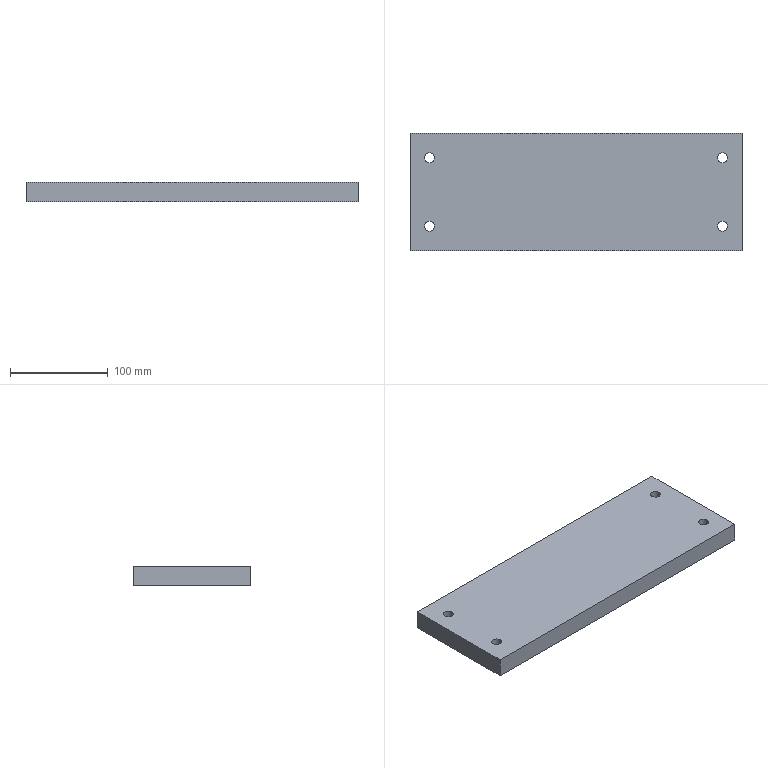Part | SolidWorks | features Extrusion 1 | 1 solid | 14 faces | box 340 x 120 x 20 mm | volume 809717 mm3 | cylinder 8 | plane 6 | commonest cylinder face diameters 10 x8
STEP:
#1=CARTESIAN_POINT('',(15.,25.,20.));
#2=VERTEX_POINT('',#1);
#3=CARTESIAN_POINT('',(25.,25.,20.));
#4=VERTEX_POINT('',#3);
#5=CARTESIAN_POINT('',(20.,25.,20.));
#6=DIRECTION('',(0.,0.,1.));
#7=DIRECTION('',(1.,0.,0.));
#8=AXIS2_PLACEMENT_3D('',#5,#6,#7);
#9=CIRCLE('',#8,5.);
#10=EDGE_CURVE('',#2,#4,#9,.T.);
#11=ORIENTED_EDGE('',*,*,#10,.T.);
#12=CARTESIAN_POINT('',(25.,25.,0.));
#13=VERTEX_POINT('',#12);
#14=CARTESIAN_POINT('',(25.,25.,20.));
#15=DIRECTION('',(0.,0.,-1.));
#16=VECTOR('',#15,1000.);
#17=LINE('',#14,#16);
#18=EDGE_CURVE('',#4,#13,#17,.T.);
#19=ORIENTED_EDGE('',*,*,#18,.T.);
#20=CARTESIAN_POINT('',(15.,25.,0.));
#21=VERTEX_POINT('',#20);
#22=CARTESIAN_POINT('',(20.,25.,0.));
#23=DIRECTION('',(0.,0.,1.));
#24=DIRECTION('',(1.,0.,0.));
#25=AXIS2_PLACEMENT_3D('',#22,#23,#24);
#26=CIRCLE('',#25,5.);
#27=EDGE_CURVE('',#21,#13,#26,.T.);
#28=ORIENTED_EDGE('',*,*,#27,.F.);
#29=CARTESIAN_POINT('',(15.,25.,20.));
#30=DIRECTION('',(0.,0.,-1.));
#31=VECTOR('',#30,1000.);
#32=LINE('',#29,#31);
#33=EDGE_CURVE('',#2,#21,#32,.T.);
#34=ORIENTED_EDGE('',*,*,#33,.F.);
#35=EDGE_LOOP('',(#11,#19,#28,#34));
#36=FACE_OUTER_BOUND('',#35,.T.);
#37=CARTESIAN_POINT('',(20.,25.,20.));
#38=DIRECTION('',(0.,0.,-1.));
#39=DIRECTION('',(-1.,0.,0.));
#40=AXIS2_PLACEMENT_3D('',#37,#38,#39);
#41=CYLINDRICAL_SURFACE('',#40,5.);
#42=ADVANCED_FACE('',(#36),#41,.F.);
#43=CARTESIAN_POINT('',(315.,25.,20.));
#44=VERTEX_POINT('',#43);
#45=CARTESIAN_POINT('',(325.,25.,20.));
#46=VERTEX_POINT('',#45);
#47=CARTESIAN_POINT('',(320.,25.,20.));
#48=DIRECTION('',(0.,0.,1.));
#49=DIRECTION('',(1.,0.,0.));
#50=AXIS2_PLACEMENT_3D('',#47,#48,#49);
#51=CIRCLE('',#50,5.);
#52=EDGE_CURVE('',#44,#46,#51,.T.);
#53=ORIENTED_EDGE('',*,*,#52,.T.);
#54=CARTESIAN_POINT('',(325.,25.,0.));
#55=VERTEX_POINT('',#54);
#56=CARTESIAN_POINT('',(325.,25.,20.));
#57=DIRECTION('',(0.,0.,-1.));
#58=VECTOR('',#57,1000.);
#59=LINE('',#56,#58);
#60=EDGE_CURVE('',#46,#55,#59,.T.);
#61=ORIENTED_EDGE('',*,*,#60,.T.);
#62=CARTESIAN_POINT('',(315.,25.,0.));
#63=VERTEX_POINT('',#62);
#64=CARTESIAN_POINT('',(320.,25.,0.));
#65=DIRECTION('',(0.,0.,1.));
#66=DIRECTION('',(1.,0.,0.));
#67=AXIS2_PLACEMENT_3D('',#64,#65,#66);
#68=CIRCLE('',#67,5.);
#69=EDGE_CURVE('',#63,#55,#68,.T.);
#70=ORIENTED_EDGE('',*,*,#69,.F.);
#71=CARTESIAN_POINT('',(315.,25.,20.));
#72=DIRECTION('',(0.,0.,-1.));
#73=VECTOR('',#72,1000.);
#74=LINE('',#71,#73);
#75=EDGE_CURVE('',#44,#63,#74,.T.);
#76=ORIENTED_EDGE('',*,*,#75,.F.);
#77=EDGE_LOOP('',(#53,#61,#70,#76));
#78=FACE_OUTER_BOUND('',#77,.T.);
#79=CARTESIAN_POINT('',(320.,25.,20.));
#80=DIRECTION('',(0.,0.,-1.));
#81=DIRECTION('',(-1.,0.,0.));
#82=AXIS2_PLACEMENT_3D('',#79,#80,#81);
#83=CYLINDRICAL_SURFACE('',#82,5.);
#84=ADVANCED_FACE('',(#78),#83,.F.);
#85=CARTESIAN_POINT('',(315.,95.,20.));
#86=VERTEX_POINT('',#85);
#87=CARTESIAN_POINT('',(325.,95.,20.));
#88=VERTEX_POINT('',#87);
#89=CARTESIAN_POINT('',(320.,95.,20.));
#90=DIRECTION('',(0.,0.,1.));
#91=DIRECTION('',(1.,0.,0.));
#92=AXIS2_PLACEMENT_3D('',#89,#90,#91);
#93=CIRCLE('',#92,5.);
#94=EDGE_CURVE('',#86,#88,#93,.T.);
#95=ORIENTED_EDGE('',*,*,#94,.T.);
#96=CARTESIAN_POINT('',(325.,95.,0.));
#97=VERTEX_POINT('',#96);
#98=CARTESIAN_POINT('',(325.,95.,20.));
#99=DIRECTION('',(0.,0.,-1.));
#100=VECTOR('',#99,1000.);
#101=LINE('',#98,#100);
#102=EDGE_CURVE('',#88,#97,#101,.T.);
#103=ORIENTED_EDGE('',*,*,#102,.T.);
#104=CARTESIAN_POINT('',(315.,95.,0.));
#105=VERTEX_POINT('',#104);
#106=CARTESIAN_POINT('',(320.,95.,0.));
#107=DIRECTION('',(0.,0.,1.));
#108=DIRECTION('',(1.,0.,0.));
#109=AXIS2_PLACEMENT_3D('',#106,#107,#108);
#110=CIRCLE('',#109,5.);
#111=EDGE_CURVE('',#105,#97,#110,.T.);
#112=ORIENTED_EDGE('',*,*,#111,.F.);
#113=CARTESIAN_POINT('',(315.,95.,20.));
#114=DIRECTION('',(0.,0.,-1.));
#115=VECTOR('',#114,1000.);
#116=LINE('',#113,#115);
#117=EDGE_CURVE('',#86,#105,#116,.T.);
#118=ORIENTED_EDGE('',*,*,#117,.F.);
#119=EDGE_LOOP('',(#95,#103,#112,#118));
#120=FACE_OUTER_BOUND('',#119,.T.);
#121=CARTESIAN_POINT('',(320.,95.,20.));
#122=DIRECTION('',(0.,0.,-1.));
#123=DIRECTION('',(-1.,0.,0.));
#124=AXIS2_PLACEMENT_3D('',#121,#122,#123);
#125=CYLINDRICAL_SURFACE('',#124,5.);
#126=ADVANCED_FACE('',(#120),#125,.F.);
#127=CARTESIAN_POINT('',(15.,95.,20.));
#128=VERTEX_POINT('',#127);
#129=CARTESIAN_POINT('',(25.,95.,20.));
#130=VERTEX_POINT('',#129);
#131=CARTESIAN_POINT('',(20.,95.,20.));
#132=DIRECTION('',(0.,0.,1.));
#133=DIRECTION('',(1.,0.,0.));
#134=AXIS2_PLACEMENT_3D('',#131,#132,#133);
#135=CIRCLE('',#134,5.);
#136=EDGE_CURVE('',#128,#130,#135,.T.);
#137=ORIENTED_EDGE('',*,*,#136,.T.);
#138=CARTESIAN_POINT('',(25.,95.,0.));
#139=VERTEX_POINT('',#138);
#140=CARTESIAN_POINT('',(25.,95.,20.));
#141=DIRECTION('',(0.,0.,-1.));
#142=VECTOR('',#141,1000.);
#143=LINE('',#140,#142);
#144=EDGE_CURVE('',#130,#139,#143,.T.);
#145=ORIENTED_EDGE('',*,*,#144,.T.);
#146=CARTESIAN_POINT('',(15.,95.,0.));
#147=VERTEX_POINT('',#146);
#148=CARTESIAN_POINT('',(20.,95.,0.));
#149=DIRECTION('',(0.,0.,1.));
#150=DIRECTION('',(1.,0.,0.));
#151=AXIS2_PLACEMENT_3D('',#148,#149,#150);
#152=CIRCLE('',#151,5.);
#153=EDGE_CURVE('',#147,#139,#152,.T.);
#154=ORIENTED_EDGE('',*,*,#153,.F.);
#155=CARTESIAN_POINT('',(15.,95.,20.));
#156=DIRECTION('',(0.,0.,-1.));
#157=VECTOR('',#156,1000.);
#158=LINE('',#155,#157);
#159=EDGE_CURVE('',#128,#147,#158,.T.);
#160=ORIENTED_EDGE('',*,*,#159,.F.);
#161=EDGE_LOOP('',(#137,#145,#154,#160));
#162=FACE_OUTER_BOUND('',#161,.T.);
#163=CARTESIAN_POINT('',(20.,95.,20.));
#164=DIRECTION('',(0.,0.,-1.));
#165=DIRECTION('',(-1.,0.,0.));
#166=AXIS2_PLACEMENT_3D('',#163,#164,#165);
#167=CYLINDRICAL_SURFACE('',#166,5.);
#168=ADVANCED_FACE('',(#162),#167,.F.);
#169=CARTESIAN_POINT('',(0.,120.,20.));
#170=VERTEX_POINT('',#169);
#171=CARTESIAN_POINT('',(0.,0.,20.));
#172=VERTEX_POINT('',#171);
#173=CARTESIAN_POINT('',(0.,0.,20.));
#174=DIRECTION('',(0.,-1.,0.));
#175=VECTOR('',#174,1000.);
#176=LINE('',#173,#175);
#177=EDGE_CURVE('',#170,#172,#176,.T.);
#178=ORIENTED_EDGE('',*,*,#177,.T.);
#179=CARTESIAN_POINT('',(340.,0.,20.));
#180=VERTEX_POINT('',#179);
#181=CARTESIAN_POINT('',(0.,0.,20.));
#182=DIRECTION('',(1.,0.,0.));
#183=VECTOR('',#182,1000.);
#184=LINE('',#181,#183);
#185=EDGE_CURVE('',#172,#180,#184,.T.);
#186=ORIENTED_EDGE('',*,*,#185,.T.);
#187=CARTESIAN_POINT('',(340.,120.,20.));
#188=VERTEX_POINT('',#187);
#189=CARTESIAN_POINT('',(340.,0.,20.));
#190=DIRECTION('',(0.,1.,0.));
#191=VECTOR('',#190,1000.);
#192=LINE('',#189,#191);
#193=EDGE_CURVE('',#180,#188,#192,.T.);
#194=ORIENTED_EDGE('',*,*,#193,.T.);
#195=CARTESIAN_POINT('',(0.,120.,20.));
#196=DIRECTION('',(-1.,0.,0.));
#197=VECTOR('',#196,1000.);
#198=LINE('',#195,#197);
#199=EDGE_CURVE('',#188,#170,#198,.T.);
#200=ORIENTED_EDGE('',*,*,#199,.T.);
#201=EDGE_LOOP('',(#178,#186,#194,#200));
#202=FACE_OUTER_BOUND('',#201,.T.);
#203=ORIENTED_EDGE('',*,*,#136,.F.);
#204=CARTESIAN_POINT('',(20.,95.,20.));
#205=DIRECTION('',(0.,0.,1.));
#206=DIRECTION('',(1.,0.,0.));
#207=AXIS2_PLACEMENT_3D('',#204,#205,#206);
#208=CIRCLE('',#207,5.);
#209=EDGE_CURVE('',#130,#128,#208,.T.);
#210=ORIENTED_EDGE('',*,*,#209,.F.);
#211=EDGE_LOOP('',(#203,#210));
#212=FACE_BOUND('',#211,.T.);
#213=ORIENTED_EDGE('',*,*,#94,.F.);
#214=CARTESIAN_POINT('',(320.,95.,20.));
#215=DIRECTION('',(0.,0.,1.));
#216=DIRECTION('',(1.,0.,0.));
#217=AXIS2_PLACEMENT_3D('',#214,#215,#216);
#218=CIRCLE('',#217,5.);
#219=EDGE_CURVE('',#88,#86,#218,.T.);
#220=ORIENTED_EDGE('',*,*,#219,.F.);
#221=EDGE_LOOP('',(#213,#220));
#222=FACE_BOUND('',#221,.T.);
#223=ORIENTED_EDGE('',*,*,#52,.F.);
#224=CARTESIAN_POINT('',(320.,25.,20.));
#225=DIRECTION('',(0.,0.,1.));
#226=DIRECTION('',(1.,0.,0.));
#227=AXIS2_PLACEMENT_3D('',#224,#225,#226);
#228=CIRCLE('',#227,5.);
#229=EDGE_CURVE('',#46,#44,#228,.T.);
#230=ORIENTED_EDGE('',*,*,#229,.F.);
#231=EDGE_LOOP('',(#223,#230));
#232=FACE_BOUND('',#231,.T.);
#233=ORIENTED_EDGE('',*,*,#10,.F.);
#234=CARTESIAN_POINT('',(20.,25.,20.));
#235=DIRECTION('',(0.,0.,1.));
#236=DIRECTION('',(1.,0.,0.));
#237=AXIS2_PLACEMENT_3D('',#234,#235,#236);
#238=CIRCLE('',#237,5.);
#239=EDGE_CURVE('',#4,#2,#238,.T.);
#240=ORIENTED_EDGE('',*,*,#239,.F.);
#241=EDGE_LOOP('',(#233,#240));
#242=FACE_BOUND('',#241,.T.);
#243=CARTESIAN_POINT('',(0.,0.,20.));
#244=DIRECTION('',(0.,0.,-1.));
#245=DIRECTION('',(-1.,0.,0.));
#246=AXIS2_PLACEMENT_3D('',#243,#244,#245);
#247=PLANE('',#246);
#248=ADVANCED_FACE('',(#202,#212,#222,#232,#242),#247,.F.);
#249=ORIENTED_EDGE('',*,*,#69,.T.);
#250=CARTESIAN_POINT('',(320.,25.,0.));
#251=DIRECTION('',(0.,0.,1.));
#252=DIRECTION('',(1.,0.,0.));
#253=AXIS2_PLACEMENT_3D('',#250,#251,#252);
#254=CIRCLE('',#253,5.);
#255=EDGE_CURVE('',#55,#63,#254,.T.);
#256=ORIENTED_EDGE('',*,*,#255,.T.);
#257=EDGE_LOOP('',(#249,#256));
#258=FACE_BOUND('',#257,.T.);
#259=ORIENTED_EDGE('',*,*,#153,.T.);
#260=CARTESIAN_POINT('',(20.,95.,0.));
#261=DIRECTION('',(0.,0.,1.));
#262=DIRECTION('',(1.,0.,0.));
#263=AXIS2_PLACEMENT_3D('',#260,#261,#262);
#264=CIRCLE('',#263,5.);
#265=EDGE_CURVE('',#139,#147,#264,.T.);
#266=ORIENTED_EDGE('',*,*,#265,.T.);
#267=EDGE_LOOP('',(#259,#266));
#268=FACE_BOUND('',#267,.T.);
#269=CARTESIAN_POINT('',(0.,120.,0.));
#270=VERTEX_POINT('',#269);
#271=CARTESIAN_POINT('',(0.,0.,0.));
#272=VERTEX_POINT('',#271);
#273=CARTESIAN_POINT('',(0.,0.,0.));
#274=DIRECTION('',(0.,-1.,0.));
#275=VECTOR('',#274,1000.);
#276=LINE('',#273,#275);
#277=EDGE_CURVE('',#270,#272,#276,.T.);
#278=ORIENTED_EDGE('',*,*,#277,.F.);
#279=CARTESIAN_POINT('',(340.,120.,0.));
#280=VERTEX_POINT('',#279);
#281=CARTESIAN_POINT('',(0.,120.,0.));
#282=DIRECTION('',(-1.,0.,0.));
#283=VECTOR('',#282,1000.);
#284=LINE('',#281,#283);
#285=EDGE_CURVE('',#280,#270,#284,.T.);
#286=ORIENTED_EDGE('',*,*,#285,.F.);
#287=CARTESIAN_POINT('',(340.,0.,0.));
#288=VERTEX_POINT('',#287);
#289=CARTESIAN_POINT('',(340.,0.,0.));
#290=DIRECTION('',(0.,1.,0.));
#291=VECTOR('',#290,1000.);
#292=LINE('',#289,#291);
#293=EDGE_CURVE('',#288,#280,#292,.T.);
#294=ORIENTED_EDGE('',*,*,#293,.F.);
#295=CARTESIAN_POINT('',(0.,0.,0.));
#296=DIRECTION('',(1.,0.,0.));
#297=VECTOR('',#296,1000.);
#298=LINE('',#295,#297);
#299=EDGE_CURVE('',#272,#288,#298,.T.);
#300=ORIENTED_EDGE('',*,*,#299,.F.);
#301=EDGE_LOOP('',(#278,#286,#294,#300));
#302=FACE_OUTER_BOUND('',#301,.T.);
#303=ORIENTED_EDGE('',*,*,#111,.T.);
#304=CARTESIAN_POINT('',(320.,95.,0.));
#305=DIRECTION('',(0.,0.,1.));
#306=DIRECTION('',(1.,0.,0.));
#307=AXIS2_PLACEMENT_3D('',#304,#305,#306);
#308=CIRCLE('',#307,5.);
#309=EDGE_CURVE('',#97,#105,#308,.T.);
#310=ORIENTED_EDGE('',*,*,#309,.T.);
#311=EDGE_LOOP('',(#303,#310));
#312=FACE_BOUND('',#311,.T.);
#313=ORIENTED_EDGE('',*,*,#27,.T.);
#314=CARTESIAN_POINT('',(20.,25.,0.));
#315=DIRECTION('',(0.,0.,1.));
#316=DIRECTION('',(1.,0.,0.));
#317=AXIS2_PLACEMENT_3D('',#314,#315,#316);
#318=CIRCLE('',#317,5.);
#319=EDGE_CURVE('',#13,#21,#318,.T.);
#320=ORIENTED_EDGE('',*,*,#319,.T.);
#321=EDGE_LOOP('',(#313,#320));
#322=FACE_BOUND('',#321,.T.);
#323=CARTESIAN_POINT('',(0.,0.,0.));
#324=DIRECTION('',(0.,0.,-1.));
#325=DIRECTION('',(-1.,0.,0.));
#326=AXIS2_PLACEMENT_3D('',#323,#324,#325);
#327=PLANE('',#326);
#328=ADVANCED_FACE('',(#258,#268,#302,#312,#322),#327,.T.);
#329=ORIENTED_EDGE('',*,*,#277,.T.);
#330=CARTESIAN_POINT('',(0.,0.,20.));
#331=DIRECTION('',(0.,0.,-1.));
#332=VECTOR('',#331,1000.);
#333=LINE('',#330,#332);
#334=EDGE_CURVE('',#172,#272,#333,.T.);
#335=ORIENTED_EDGE('',*,*,#334,.F.);
#336=ORIENTED_EDGE('',*,*,#177,.F.);
#337=CARTESIAN_POINT('',(0.,120.,20.));
#338=DIRECTION('',(0.,0.,-1.));
#339=VECTOR('',#338,1000.);
#340=LINE('',#337,#339);
#341=EDGE_CURVE('',#170,#270,#340,.T.);
#342=ORIENTED_EDGE('',*,*,#341,.T.);
#343=EDGE_LOOP('',(#329,#335,#336,#342));
#344=FACE_OUTER_BOUND('',#343,.T.);
#345=CARTESIAN_POINT('',(0.,0.,20.));
#346=DIRECTION('',(1.,0.,0.));
#347=DIRECTION('',(0.,0.,-1.));
#348=AXIS2_PLACEMENT_3D('',#345,#346,#347);
#349=PLANE('',#348);
#350=ADVANCED_FACE('',(#344),#349,.F.);
#351=ORIENTED_EDGE('',*,*,#299,.T.);
#352=CARTESIAN_POINT('',(340.,0.,20.));
#353=DIRECTION('',(0.,0.,-1.));
#354=VECTOR('',#353,1000.);
#355=LINE('',#352,#354);
#356=EDGE_CURVE('',#180,#288,#355,.T.);
#357=ORIENTED_EDGE('',*,*,#356,.F.);
#358=ORIENTED_EDGE('',*,*,#185,.F.);
#359=ORIENTED_EDGE('',*,*,#334,.T.);
#360=EDGE_LOOP('',(#351,#357,#358,#359));
#361=FACE_OUTER_BOUND('',#360,.T.);
#362=CARTESIAN_POINT('',(0.,0.,20.));
#363=DIRECTION('',(0.,1.,0.));
#364=DIRECTION('',(0.,0.,1.));
#365=AXIS2_PLACEMENT_3D('',#362,#363,#364);
#366=PLANE('',#365);
#367=ADVANCED_FACE('',(#361),#366,.F.);
#368=ORIENTED_EDGE('',*,*,#293,.T.);
#369=CARTESIAN_POINT('',(340.,120.,20.));
#370=DIRECTION('',(0.,0.,-1.));
#371=VECTOR('',#370,1000.);
#372=LINE('',#369,#371);
#373=EDGE_CURVE('',#188,#280,#372,.T.);
#374=ORIENTED_EDGE('',*,*,#373,.F.);
#375=ORIENTED_EDGE('',*,*,#193,.F.);
#376=ORIENTED_EDGE('',*,*,#356,.T.);
#377=EDGE_LOOP('',(#368,#374,#375,#376));
#378=FACE_OUTER_BOUND('',#377,.T.);
#379=CARTESIAN_POINT('',(340.,0.,20.));
#380=DIRECTION('',(-1.,0.,0.));
#381=DIRECTION('',(0.,0.,1.));
#382=AXIS2_PLACEMENT_3D('',#379,#380,#381);
#383=PLANE('',#382);
#384=ADVANCED_FACE('',(#378),#383,.F.);
#385=ORIENTED_EDGE('',*,*,#285,.T.);
#386=ORIENTED_EDGE('',*,*,#341,.F.);
#387=ORIENTED_EDGE('',*,*,#199,.F.);
#388=ORIENTED_EDGE('',*,*,#373,.T.);
#389=EDGE_LOOP('',(#385,#386,#387,#388));
#390=FACE_OUTER_BOUND('',#389,.T.);
#391=CARTESIAN_POINT('',(0.,120.,20.));
#392=DIRECTION('',(0.,-1.,0.));
#393=DIRECTION('',(0.,0.,-1.));
#394=AXIS2_PLACEMENT_3D('',#391,#392,#393);
#395=PLANE('',#394);
#396=ADVANCED_FACE('',(#390),#395,.F.);
#397=ORIENTED_EDGE('',*,*,#144,.F.);
#398=ORIENTED_EDGE('',*,*,#209,.T.);
#399=ORIENTED_EDGE('',*,*,#159,.T.);
#400=ORIENTED_EDGE('',*,*,#265,.F.);
#401=EDGE_LOOP('',(#397,#398,#399,#400));
#402=FACE_OUTER_BOUND('',#401,.T.);
#403=CARTESIAN_POINT('',(20.,95.,20.));
#404=DIRECTION('',(0.,0.,-1.));
#405=DIRECTION('',(-1.,0.,0.));
#406=AXIS2_PLACEMENT_3D('',#403,#404,#405);
#407=CYLINDRICAL_SURFACE('',#406,5.);
#408=ADVANCED_FACE('',(#402),#407,.F.);
#409=ORIENTED_EDGE('',*,*,#102,.F.);
#410=ORIENTED_EDGE('',*,*,#219,.T.);
#411=ORIENTED_EDGE('',*,*,#117,.T.);
#412=ORIENTED_EDGE('',*,*,#309,.F.);
#413=EDGE_LOOP('',(#409,#410,#411,#412));
#414=FACE_OUTER_BOUND('',#413,.T.);
#415=CARTESIAN_POINT('',(320.,95.,20.));
#416=DIRECTION('',(0.,0.,-1.));
#417=DIRECTION('',(-1.,0.,0.));
#418=AXIS2_PLACEMENT_3D('',#415,#416,#417);
#419=CYLINDRICAL_SURFACE('',#418,5.);
#420=ADVANCED_FACE('',(#414),#419,.F.);
#421=ORIENTED_EDGE('',*,*,#60,.F.);
#422=ORIENTED_EDGE('',*,*,#229,.T.);
#423=ORIENTED_EDGE('',*,*,#75,.T.);
#424=ORIENTED_EDGE('',*,*,#255,.F.);
#425=EDGE_LOOP('',(#421,#422,#423,#424));
#426=FACE_OUTER_BOUND('',#425,.T.);
#427=CARTESIAN_POINT('',(320.,25.,20.));
#428=DIRECTION('',(0.,0.,-1.));
#429=DIRECTION('',(-1.,0.,0.));
#430=AXIS2_PLACEMENT_3D('',#427,#428,#429);
#431=CYLINDRICAL_SURFACE('',#430,5.);
#432=ADVANCED_FACE('',(#426),#431,.F.);
#433=ORIENTED_EDGE('',*,*,#18,.F.);
#434=ORIENTED_EDGE('',*,*,#239,.T.);
#435=ORIENTED_EDGE('',*,*,#33,.T.);
#436=ORIENTED_EDGE('',*,*,#319,.F.);
#437=EDGE_LOOP('',(#433,#434,#435,#436));
#438=FACE_OUTER_BOUND('',#437,.T.);
#439=CARTESIAN_POINT('',(20.,25.,20.));
#440=DIRECTION('',(0.,0.,-1.));
#441=DIRECTION('',(-1.,0.,0.));
#442=AXIS2_PLACEMENT_3D('',#439,#440,#441);
#443=CYLINDRICAL_SURFACE('',#442,5.);
#444=ADVANCED_FACE('',(#438),#443,.F.);
#445=CLOSED_SHELL('',(#42,#84,#126,#168,#248,#328,#350,#367,#384,#396,#408,#420,#432,#444));
#446=MANIFOLD_SOLID_BREP('',#445);
#447=CARTESIAN_POINT('',(0.,0.,0.));
#448=DIRECTION('',(0.,0.,1.));
#449=DIRECTION('',(1.,0.,0.));
#450=AXIS2_PLACEMENT_3D('',#447,#448,#449);
#451=(LENGTH_UNIT()NAMED_UNIT(*)SI_UNIT(.MILLI.,.METRE.));
#452=UNCERTAINTY_MEASURE_WITH_UNIT(LENGTH_MEASURE(0.00001),#451,'','');
#453=(NAMED_UNIT(*)PLANE_ANGLE_UNIT()SI_UNIT($,.RADIAN.));
#454=(NAMED_UNIT(*)SI_UNIT($,.STERADIAN.)SOLID_ANGLE_UNIT());
#455=(GEOMETRIC_REPRESENTATION_CONTEXT(3)GLOBAL_UNCERTAINTY_ASSIGNED_CONTEXT((#452))GLOBAL_UNIT_ASSIGNED_CONTEXT((#451,#453,#454))REPRESENTATION_CONTEXT('',''));
#456=ADVANCED_BREP_SHAPE_REPRESENTATION('',(#446,#450),#455);